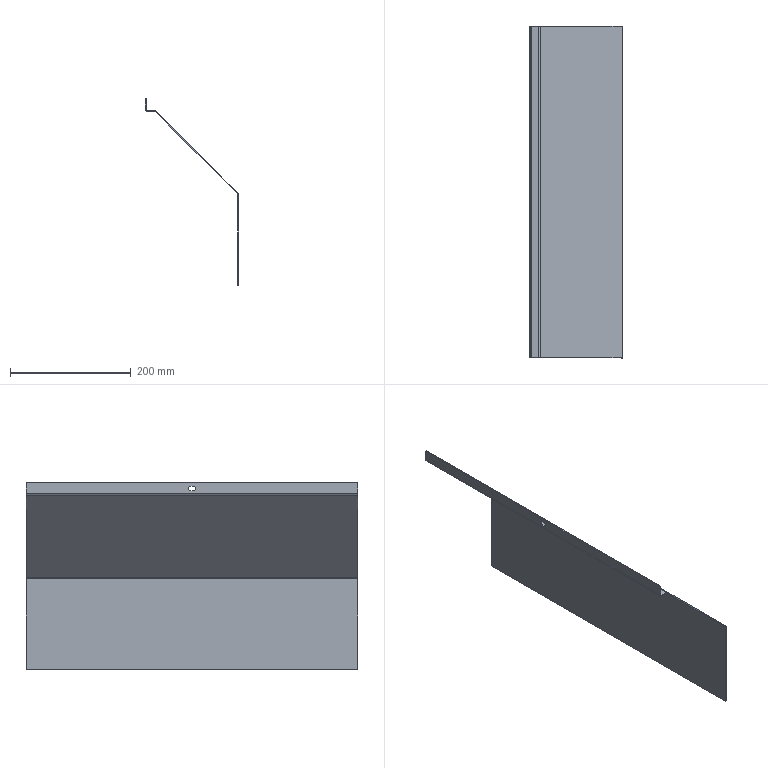Part | STEP file | SYL_0392D6J1SYL0380DJ100-939135 | 1 solid | 34 faces | box 155 x 550 x 310 mm | volume 314616 mm3 | plane 26 | cylinder 8 | commonest cylinder face diameters 4 x3 7 x3 8 x2
STEP:
#1=CARTESIAN_POINT('',(-1.5,-2.,14.));
#2=VERTEX_POINT('',#1);
#3=CARTESIAN_POINT('',(0.,-2.,14.));
#4=VERTEX_POINT('',#3);
#5=CARTESIAN_POINT('',(0.,-2.,14.));
#6=DIRECTION('',(1.,0.,0.));
#7=VECTOR('',#6,1000.);
#8=LINE('',#5,#7);
#9=EDGE_CURVE('',#2,#4,#8,.T.);
#10=ORIENTED_EDGE('',*,*,#9,.F.);
#11=CARTESIAN_POINT('',(-1.5,2.,14.));
#12=VERTEX_POINT('',#11);
#13=CARTESIAN_POINT('',(-1.5,-275.,14.));
#14=DIRECTION('',(0.,-1.,0.));
#15=VECTOR('',#14,1000.);
#16=LINE('',#13,#15);
#17=EDGE_CURVE('',#12,#2,#16,.T.);
#18=ORIENTED_EDGE('',*,*,#17,.F.);
#19=CARTESIAN_POINT('',(0.,2.,14.));
#20=VERTEX_POINT('',#19);
#21=CARTESIAN_POINT('',(0.,2.,14.));
#22=DIRECTION('',(1.,0.,0.));
#23=VECTOR('',#22,1000.);
#24=LINE('',#21,#23);
#25=EDGE_CURVE('',#12,#20,#24,.T.);
#26=ORIENTED_EDGE('',*,*,#25,.T.);
#27=CARTESIAN_POINT('',(0.,2.,14.));
#28=DIRECTION('',(0.,-1.,0.));
#29=VECTOR('',#28,1000.);
#30=LINE('',#27,#29);
#31=EDGE_CURVE('',#20,#4,#30,.T.);
#32=ORIENTED_EDGE('',*,*,#31,.T.);
#33=EDGE_LOOP('',(#10,#18,#26,#32));
#34=FACE_OUTER_BOUND('',#33,.T.);
#35=CARTESIAN_POINT('',(0.,2.,14.));
#36=DIRECTION('',(0.,0.,1.));
#37=DIRECTION('',(0.,-1.,0.));
#38=AXIS2_PLACEMENT_3D('',#35,#36,#37);
#39=PLANE('',#38);
#40=ADVANCED_FACE('',(#34),#39,.F.);
#41=ORIENTED_EDGE('',*,*,#25,.F.);
#42=CARTESIAN_POINT('',(-1.5,2.,6.));
#43=VERTEX_POINT('',#42);
#44=CARTESIAN_POINT('',(-1.5,2.,10.));
#45=DIRECTION('',(-1.,0.,0.));
#46=DIRECTION('',(0.,0.,1.));
#47=AXIS2_PLACEMENT_3D('',#44,#45,#46);
#48=CIRCLE('',#47,4.);
#49=EDGE_CURVE('',#12,#43,#48,.T.);
#50=ORIENTED_EDGE('',*,*,#49,.T.);
#51=CARTESIAN_POINT('',(0.,2.,6.));
#52=VERTEX_POINT('',#51);
#53=CARTESIAN_POINT('',(0.,2.,6.));
#54=DIRECTION('',(1.,0.,0.));
#55=VECTOR('',#54,1000.);
#56=LINE('',#53,#55);
#57=EDGE_CURVE('',#43,#52,#56,.T.);
#58=ORIENTED_EDGE('',*,*,#57,.T.);
#59=CARTESIAN_POINT('',(0.,2.,10.));
#60=DIRECTION('',(-1.,0.,0.));
#61=DIRECTION('',(0.,0.,1.));
#62=AXIS2_PLACEMENT_3D('',#59,#60,#61);
#63=CIRCLE('',#62,4.);
#64=EDGE_CURVE('',#20,#52,#63,.T.);
#65=ORIENTED_EDGE('',*,*,#64,.F.);
#66=EDGE_LOOP('',(#41,#50,#58,#65));
#67=FACE_OUTER_BOUND('',#66,.T.);
#68=CARTESIAN_POINT('',(0.,2.,10.));
#69=DIRECTION('',(1.,0.,0.));
#70=DIRECTION('',(0.,0.,-1.));
#71=AXIS2_PLACEMENT_3D('',#68,#69,#70);
#72=CYLINDRICAL_SURFACE('',#71,4.);
#73=ADVANCED_FACE('',(#67),#72,.F.);
#74=ORIENTED_EDGE('',*,*,#57,.F.);
#75=CARTESIAN_POINT('',(-1.5,-2.,6.));
#76=VERTEX_POINT('',#75);
#77=CARTESIAN_POINT('',(-1.5,-275.,6.));
#78=DIRECTION('',(0.,1.,0.));
#79=VECTOR('',#78,1000.);
#80=LINE('',#77,#79);
#81=EDGE_CURVE('',#76,#43,#80,.T.);
#82=ORIENTED_EDGE('',*,*,#81,.F.);
#83=CARTESIAN_POINT('',(0.,-2.,6.));
#84=VERTEX_POINT('',#83);
#85=CARTESIAN_POINT('',(0.,-2.,6.));
#86=DIRECTION('',(1.,0.,0.));
#87=VECTOR('',#86,1000.);
#88=LINE('',#85,#87);
#89=EDGE_CURVE('',#76,#84,#88,.T.);
#90=ORIENTED_EDGE('',*,*,#89,.T.);
#91=CARTESIAN_POINT('',(0.,-2.,6.));
#92=DIRECTION('',(0.,1.,0.));
#93=VECTOR('',#92,1000.);
#94=LINE('',#91,#93);
#95=EDGE_CURVE('',#84,#52,#94,.T.);
#96=ORIENTED_EDGE('',*,*,#95,.T.);
#97=EDGE_LOOP('',(#74,#82,#90,#96));
#98=FACE_OUTER_BOUND('',#97,.T.);
#99=CARTESIAN_POINT('',(0.,-2.,6.));
#100=DIRECTION('',(0.,0.,-1.));
#101=DIRECTION('',(0.,1.,0.));
#102=AXIS2_PLACEMENT_3D('',#99,#100,#101);
#103=PLANE('',#102);
#104=ADVANCED_FACE('',(#98),#103,.F.);
#105=CARTESIAN_POINT('',(14.05,-275.,-1.5));
#106=VERTEX_POINT('',#105);
#107=CARTESIAN_POINT('',(14.05,-275.,0.));
#108=VERTEX_POINT('',#107);
#109=CARTESIAN_POINT('',(14.05,-275.,0.));
#110=DIRECTION('',(0.,0.,1.));
#111=VECTOR('',#110,1000.);
#112=LINE('',#109,#111);
#113=EDGE_CURVE('',#106,#108,#112,.T.);
#114=ORIENTED_EDGE('',*,*,#113,.F.);
#115=CARTESIAN_POINT('',(15.464,-275.,-2.086));
#116=VERTEX_POINT('',#115);
#117=CARTESIAN_POINT('',(14.05,-275.,-3.5));
#118=DIRECTION('',(0.,-1.,0.));
#119=DIRECTION('',(0.,0.,-1.));
#120=AXIS2_PLACEMENT_3D('',#117,#118,#119);
#121=CIRCLE('',#120,2.);
#122=EDGE_CURVE('',#116,#106,#121,.T.);
#123=ORIENTED_EDGE('',*,*,#122,.F.);
#124=CARTESIAN_POINT('',(16.525,-275.,-1.025));
#125=VERTEX_POINT('',#124);
#126=CARTESIAN_POINT('',(16.525,-275.,-1.025));
#127=DIRECTION('',(0.7071,0.,0.7071));
#128=VECTOR('',#127,1000.);
#129=LINE('',#126,#128);
#130=EDGE_CURVE('',#116,#125,#129,.T.);
#131=ORIENTED_EDGE('',*,*,#130,.T.);
#132=CARTESIAN_POINT('',(14.05,-275.,-3.5));
#133=DIRECTION('',(0.,-1.,0.));
#134=DIRECTION('',(0.7071,0.,0.7071));
#135=AXIS2_PLACEMENT_3D('',#132,#133,#134);
#136=CIRCLE('',#135,3.5);
#137=EDGE_CURVE('',#125,#108,#136,.T.);
#138=ORIENTED_EDGE('',*,*,#137,.T.);
#139=EDGE_LOOP('',(#114,#123,#131,#138));
#140=FACE_OUTER_BOUND('',#139,.T.);
#141=CARTESIAN_POINT('',(14.05,-275.,-3.5));
#142=DIRECTION('',(0.,1.,0.));
#143=DIRECTION('',(0.,0.,1.));
#144=AXIS2_PLACEMENT_3D('',#141,#142,#143);
#145=PLANE('',#144);
#146=ADVANCED_FACE('',(#140),#145,.F.);
#147=ORIENTED_EDGE('',*,*,#130,.F.);
#148=CARTESIAN_POINT('',(151.414,-275.,-138.036));
#149=VERTEX_POINT('',#148);
#150=CARTESIAN_POINT('',(14.439,-275.,-1.061));
#151=DIRECTION('',(-0.7071,0.,0.7071));
#152=VECTOR('',#151,1000.);
#153=LINE('',#150,#152);
#154=EDGE_CURVE('',#149,#116,#153,.T.);
#155=ORIENTED_EDGE('',*,*,#154,.F.);
#156=CARTESIAN_POINT('',(152.475,-275.,-136.975));
#157=VERTEX_POINT('',#156);
#158=CARTESIAN_POINT('',(152.475,-275.,-136.975));
#159=DIRECTION('',(0.7071,0.,0.7071));
#160=VECTOR('',#159,1000.);
#161=LINE('',#158,#160);
#162=EDGE_CURVE('',#149,#157,#161,.T.);
#163=ORIENTED_EDGE('',*,*,#162,.T.);
#164=CARTESIAN_POINT('',(152.475,-275.,-136.975));
#165=DIRECTION('',(-0.7071,0.,0.7071));
#166=VECTOR('',#165,1000.);
#167=LINE('',#164,#166);
#168=EDGE_CURVE('',#157,#125,#167,.T.);
#169=ORIENTED_EDGE('',*,*,#168,.T.);
#170=EDGE_LOOP('',(#147,#155,#163,#169));
#171=FACE_OUTER_BOUND('',#170,.T.);
#172=CARTESIAN_POINT('',(152.475,-275.,-136.975));
#173=DIRECTION('',(0.,1.,0.));
#174=DIRECTION('',(-0.7071,0.,0.7071));
#175=AXIS2_PLACEMENT_3D('',#172,#173,#174);
#176=PLANE('',#175);
#177=ADVANCED_FACE('',(#171),#176,.F.);
#178=ORIENTED_EDGE('',*,*,#162,.F.);
#179=CARTESIAN_POINT('',(152.,-275.,-139.45));
#180=VERTEX_POINT('',#179);
#181=CARTESIAN_POINT('',(150.,-275.,-139.45));
#182=DIRECTION('',(0.,-1.,0.));
#183=DIRECTION('',(0.,0.,-1.));
#184=AXIS2_PLACEMENT_3D('',#181,#182,#183);
#185=CIRCLE('',#184,2.);
#186=EDGE_CURVE('',#180,#149,#185,.T.);
#187=ORIENTED_EDGE('',*,*,#186,.F.);
#188=CARTESIAN_POINT('',(153.5,-275.,-139.45));
#189=VERTEX_POINT('',#188);
#190=CARTESIAN_POINT('',(153.5,-275.,-139.45));
#191=DIRECTION('',(1.,0.,0.));
#192=VECTOR('',#191,1000.);
#193=LINE('',#190,#192);
#194=EDGE_CURVE('',#180,#189,#193,.T.);
#195=ORIENTED_EDGE('',*,*,#194,.T.);
#196=CARTESIAN_POINT('',(150.,-275.,-139.45));
#197=DIRECTION('',(0.,-1.,0.));
#198=DIRECTION('',(1.,0.,0.));
#199=AXIS2_PLACEMENT_3D('',#196,#197,#198);
#200=CIRCLE('',#199,3.5);
#201=EDGE_CURVE('',#189,#157,#200,.T.);
#202=ORIENTED_EDGE('',*,*,#201,.T.);
#203=EDGE_LOOP('',(#178,#187,#195,#202));
#204=FACE_OUTER_BOUND('',#203,.T.);
#205=CARTESIAN_POINT('',(150.,-275.,-139.45));
#206=DIRECTION('',(0.,1.,0.));
#207=DIRECTION('',(0.,0.,1.));
#208=AXIS2_PLACEMENT_3D('',#205,#206,#207);
#209=PLANE('',#208);
#210=ADVANCED_FACE('',(#204),#209,.F.);
#211=ORIENTED_EDGE('',*,*,#194,.F.);
#212=CARTESIAN_POINT('',(152.,-275.,-290.));
#213=VERTEX_POINT('',#212);
#214=CARTESIAN_POINT('',(152.,-275.,-138.));
#215=DIRECTION('',(0.,0.,1.));
#216=VECTOR('',#215,1000.);
#217=LINE('',#214,#216);
#218=EDGE_CURVE('',#213,#180,#217,.T.);
#219=ORIENTED_EDGE('',*,*,#218,.F.);
#220=CARTESIAN_POINT('',(153.5,-275.,-290.));
#221=VERTEX_POINT('',#220);
#222=CARTESIAN_POINT('',(153.5,-275.,-290.));
#223=DIRECTION('',(1.,0.,0.));
#224=VECTOR('',#223,1000.);
#225=LINE('',#222,#224);
#226=EDGE_CURVE('',#213,#221,#225,.T.);
#227=ORIENTED_EDGE('',*,*,#226,.T.);
#228=CARTESIAN_POINT('',(153.5,-275.,-290.));
#229=DIRECTION('',(0.,0.,1.));
#230=VECTOR('',#229,1000.);
#231=LINE('',#228,#230);
#232=EDGE_CURVE('',#221,#189,#231,.T.);
#233=ORIENTED_EDGE('',*,*,#232,.T.);
#234=EDGE_LOOP('',(#211,#219,#227,#233));
#235=FACE_OUTER_BOUND('',#234,.T.);
#236=CARTESIAN_POINT('',(153.5,-275.,-290.));
#237=DIRECTION('',(0.,1.,0.));
#238=DIRECTION('',(0.,0.,1.));
#239=AXIS2_PLACEMENT_3D('',#236,#237,#238);
#240=PLANE('',#239);
#241=ADVANCED_FACE('',(#235),#240,.F.);
#242=ORIENTED_EDGE('',*,*,#226,.F.);
#243=CARTESIAN_POINT('',(152.,275.,-290.));
#244=VERTEX_POINT('',#243);
#245=CARTESIAN_POINT('',(152.,-275.,-290.));
#246=DIRECTION('',(0.,-1.,0.));
#247=VECTOR('',#246,1000.);
#248=LINE('',#245,#247);
#249=EDGE_CURVE('',#244,#213,#248,.T.);
#250=ORIENTED_EDGE('',*,*,#249,.F.);
#251=CARTESIAN_POINT('',(153.5,275.,-290.));
#252=VERTEX_POINT('',#251);
#253=CARTESIAN_POINT('',(153.5,275.,-290.));
#254=DIRECTION('',(1.,0.,0.));
#255=VECTOR('',#254,1000.);
#256=LINE('',#253,#255);
#257=EDGE_CURVE('',#244,#252,#256,.T.);
#258=ORIENTED_EDGE('',*,*,#257,.T.);
#259=CARTESIAN_POINT('',(153.5,275.,-290.));
#260=DIRECTION('',(0.,-1.,0.));
#261=VECTOR('',#260,1000.);
#262=LINE('',#259,#261);
#263=EDGE_CURVE('',#252,#221,#262,.T.);
#264=ORIENTED_EDGE('',*,*,#263,.T.);
#265=EDGE_LOOP('',(#242,#250,#258,#264));
#266=FACE_OUTER_BOUND('',#265,.T.);
#267=CARTESIAN_POINT('',(153.5,275.,-290.));
#268=DIRECTION('',(0.,0.,1.));
#269=DIRECTION('',(0.,-1.,0.));
#270=AXIS2_PLACEMENT_3D('',#267,#268,#269);
#271=PLANE('',#270);
#272=ADVANCED_FACE('',(#266),#271,.F.);
#273=ORIENTED_EDGE('',*,*,#257,.F.);
#274=CARTESIAN_POINT('',(152.,275.,-139.45));
#275=VERTEX_POINT('',#274);
#276=CARTESIAN_POINT('',(152.,275.,-138.));
#277=DIRECTION('',(0.,0.,-1.));
#278=VECTOR('',#277,1000.);
#279=LINE('',#276,#278);
#280=EDGE_CURVE('',#275,#244,#279,.T.);
#281=ORIENTED_EDGE('',*,*,#280,.F.);
#282=CARTESIAN_POINT('',(153.5,275.,-139.45));
#283=VERTEX_POINT('',#282);
#284=CARTESIAN_POINT('',(153.5,275.,-139.45));
#285=DIRECTION('',(1.,0.,0.));
#286=VECTOR('',#285,1000.);
#287=LINE('',#284,#286);
#288=EDGE_CURVE('',#275,#283,#287,.T.);
#289=ORIENTED_EDGE('',*,*,#288,.T.);
#290=CARTESIAN_POINT('',(153.5,275.,-139.45));
#291=DIRECTION('',(0.,0.,-1.));
#292=VECTOR('',#291,1000.);
#293=LINE('',#290,#292);
#294=EDGE_CURVE('',#283,#252,#293,.T.);
#295=ORIENTED_EDGE('',*,*,#294,.T.);
#296=EDGE_LOOP('',(#273,#281,#289,#295));
#297=FACE_OUTER_BOUND('',#296,.T.);
#298=CARTESIAN_POINT('',(153.5,275.,-139.45));
#299=DIRECTION('',(0.,-1.,0.));
#300=DIRECTION('',(0.,0.,-1.));
#301=AXIS2_PLACEMENT_3D('',#298,#299,#300);
#302=PLANE('',#301);
#303=ADVANCED_FACE('',(#297),#302,.F.);
#304=ORIENTED_EDGE('',*,*,#288,.F.);
#305=CARTESIAN_POINT('',(151.414,275.,-138.036));
#306=VERTEX_POINT('',#305);
#307=CARTESIAN_POINT('',(150.,275.,-139.45));
#308=DIRECTION('',(0.,1.,0.));
#309=DIRECTION('',(0.,0.,-1.));
#310=AXIS2_PLACEMENT_3D('',#307,#308,#309);
#311=CIRCLE('',#310,2.);
#312=EDGE_CURVE('',#306,#275,#311,.T.);
#313=ORIENTED_EDGE('',*,*,#312,.F.);
#314=CARTESIAN_POINT('',(152.475,275.,-136.975));
#315=VERTEX_POINT('',#314);
#316=CARTESIAN_POINT('',(152.475,275.,-136.975));
#317=DIRECTION('',(0.7071,0.,0.7071));
#318=VECTOR('',#317,1000.);
#319=LINE('',#316,#318);
#320=EDGE_CURVE('',#306,#315,#319,.T.);
#321=ORIENTED_EDGE('',*,*,#320,.T.);
#322=CARTESIAN_POINT('',(150.,275.,-139.45));
#323=DIRECTION('',(0.,1.,0.));
#324=DIRECTION('',(0.7071,0.,0.7071));
#325=AXIS2_PLACEMENT_3D('',#322,#323,#324);
#326=CIRCLE('',#325,3.5);
#327=EDGE_CURVE('',#315,#283,#326,.T.);
#328=ORIENTED_EDGE('',*,*,#327,.T.);
#329=EDGE_LOOP('',(#304,#313,#321,#328));
#330=FACE_OUTER_BOUND('',#329,.T.);
#331=CARTESIAN_POINT('',(150.,275.,-139.45));
#332=DIRECTION('',(0.,-1.,0.));
#333=DIRECTION('',(0.,0.,-1.));
#334=AXIS2_PLACEMENT_3D('',#331,#332,#333);
#335=PLANE('',#334);
#336=ADVANCED_FACE('',(#330),#335,.F.);
#337=ORIENTED_EDGE('',*,*,#320,.F.);
#338=CARTESIAN_POINT('',(15.464,275.,-2.086));
#339=VERTEX_POINT('',#338);
#340=CARTESIAN_POINT('',(14.439,275.,-1.061));
#341=DIRECTION('',(0.7071,0.,-0.7071));
#342=VECTOR('',#341,1000.);
#343=LINE('',#340,#342);
#344=EDGE_CURVE('',#339,#306,#343,.T.);
#345=ORIENTED_EDGE('',*,*,#344,.F.);
#346=CARTESIAN_POINT('',(16.525,275.,-1.025));
#347=VERTEX_POINT('',#346);
#348=CARTESIAN_POINT('',(16.525,275.,-1.025));
#349=DIRECTION('',(0.7071,0.,0.7071));
#350=VECTOR('',#349,1000.);
#351=LINE('',#348,#350);
#352=EDGE_CURVE('',#339,#347,#351,.T.);
#353=ORIENTED_EDGE('',*,*,#352,.T.);
#354=CARTESIAN_POINT('',(16.525,275.,-1.025));
#355=DIRECTION('',(0.7071,0.,-0.7071));
#356=VECTOR('',#355,1000.);
#357=LINE('',#354,#356);
#358=EDGE_CURVE('',#347,#315,#357,.T.);
#359=ORIENTED_EDGE('',*,*,#358,.T.);
#360=EDGE_LOOP('',(#337,#345,#353,#359));
#361=FACE_OUTER_BOUND('',#360,.T.);
#362=CARTESIAN_POINT('',(16.525,275.,-1.025));
#363=DIRECTION('',(0.,-1.,0.));
#364=DIRECTION('',(0.7071,0.,-0.7071));
#365=AXIS2_PLACEMENT_3D('',#362,#363,#364);
#366=PLANE('',#365);
#367=ADVANCED_FACE('',(#361),#366,.F.);
#368=ORIENTED_EDGE('',*,*,#352,.F.);
#369=CARTESIAN_POINT('',(14.05,275.,-1.5));
#370=VERTEX_POINT('',#369);
#371=CARTESIAN_POINT('',(14.05,275.,-3.5));
#372=DIRECTION('',(0.,1.,0.));
#373=DIRECTION('',(0.,0.,-1.));
#374=AXIS2_PLACEMENT_3D('',#371,#372,#373);
#375=CIRCLE('',#374,2.);
#376=EDGE_CURVE('',#370,#339,#375,.T.);
#377=ORIENTED_EDGE('',*,*,#376,.F.);
#378=CARTESIAN_POINT('',(14.05,275.,0.));
#379=VERTEX_POINT('',#378);
#380=CARTESIAN_POINT('',(14.05,275.,0.));
#381=DIRECTION('',(0.,0.,1.));
#382=VECTOR('',#381,1000.);
#383=LINE('',#380,#382);
#384=EDGE_CURVE('',#370,#379,#383,.T.);
#385=ORIENTED_EDGE('',*,*,#384,.T.);
#386=CARTESIAN_POINT('',(14.05,275.,-3.5));
#387=DIRECTION('',(0.,1.,0.));
#388=DIRECTION('',(0.,0.,1.));
#389=AXIS2_PLACEMENT_3D('',#386,#387,#388);
#390=CIRCLE('',#389,3.5);
#391=EDGE_CURVE('',#379,#347,#390,.T.);
#392=ORIENTED_EDGE('',*,*,#391,.T.);
#393=EDGE_LOOP('',(#368,#377,#385,#392));
#394=FACE_OUTER_BOUND('',#393,.T.);
#395=CARTESIAN_POINT('',(14.05,275.,-3.5));
#396=DIRECTION('',(0.,-1.,0.));
#397=DIRECTION('',(0.,0.,-1.));
#398=AXIS2_PLACEMENT_3D('',#395,#396,#397);
#399=PLANE('',#398);
#400=ADVANCED_FACE('',(#394),#399,.F.);
#401=ORIENTED_EDGE('',*,*,#384,.F.);
#402=CARTESIAN_POINT('',(2.,275.,-1.5));
#403=VERTEX_POINT('',#402);
#404=CARTESIAN_POINT('',(0.,275.,-1.5));
#405=DIRECTION('',(1.,0.,0.));
#406=VECTOR('',#405,1000.);
#407=LINE('',#404,#406);
#408=EDGE_CURVE('',#403,#370,#407,.T.);
#409=ORIENTED_EDGE('',*,*,#408,.F.);
#410=CARTESIAN_POINT('',(2.,275.,0.));
#411=VERTEX_POINT('',#410);
#412=CARTESIAN_POINT('',(2.,275.,0.));
#413=DIRECTION('',(0.,0.,1.));
#414=VECTOR('',#413,1000.);
#415=LINE('',#412,#414);
#416=EDGE_CURVE('',#403,#411,#415,.T.);
#417=ORIENTED_EDGE('',*,*,#416,.T.);
#418=CARTESIAN_POINT('',(2.,275.,0.));
#419=DIRECTION('',(1.,0.,0.));
#420=VECTOR('',#419,1000.);
#421=LINE('',#418,#420);
#422=EDGE_CURVE('',#411,#379,#421,.T.);
#423=ORIENTED_EDGE('',*,*,#422,.T.);
#424=EDGE_LOOP('',(#401,#409,#417,#423));
#425=FACE_OUTER_BOUND('',#424,.T.);
#426=CARTESIAN_POINT('',(2.,275.,0.));
#427=DIRECTION('',(0.,-1.,0.));
#428=DIRECTION('',(1.,0.,0.));
#429=AXIS2_PLACEMENT_3D('',#426,#427,#428);
#430=PLANE('',#429);
#431=ADVANCED_FACE('',(#425),#430,.F.);
#432=ORIENTED_EDGE('',*,*,#416,.F.);
#433=CARTESIAN_POINT('',(-1.5,275.,2.));
#434=VERTEX_POINT('',#433);
#435=CARTESIAN_POINT('',(2.,275.,2.));
#436=DIRECTION('',(0.,-1.,0.));
#437=DIRECTION('',(0.,0.,1.));
#438=AXIS2_PLACEMENT_3D('',#435,#436,#437);
#439=CIRCLE('',#438,3.5);
#440=EDGE_CURVE('',#434,#403,#439,.T.);
#441=ORIENTED_EDGE('',*,*,#440,.F.);
#442=CARTESIAN_POINT('',(0.,275.,2.));
#443=VERTEX_POINT('',#442);
#444=CARTESIAN_POINT('',(0.,275.,2.));
#445=DIRECTION('',(1.,0.,0.));
#446=VECTOR('',#445,1000.);
#447=LINE('',#444,#446);
#448=EDGE_CURVE('',#434,#443,#447,.T.);
#449=ORIENTED_EDGE('',*,*,#448,.T.);
#450=CARTESIAN_POINT('',(2.,275.,2.));
#451=DIRECTION('',(0.,-1.,0.));
#452=DIRECTION('',(-1.,0.,0.));
#453=AXIS2_PLACEMENT_3D('',#450,#451,#452);
#454=CIRCLE('',#453,2.);
#455=EDGE_CURVE('',#443,#411,#454,.T.);
#456=ORIENTED_EDGE('',*,*,#455,.T.);
#457=EDGE_LOOP('',(#432,#441,#449,#456));
#458=FACE_OUTER_BOUND('',#457,.T.);
#459=CARTESIAN_POINT('',(2.,275.,2.));
#460=DIRECTION('',(0.,1.,0.));
#461=DIRECTION('',(0.,0.,1.));
#462=AXIS2_PLACEMENT_3D('',#459,#460,#461);
#463=PLANE('',#462);
#464=ADVANCED_FACE('',(#458),#463,.T.);
#465=ORIENTED_EDGE('',*,*,#448,.F.);
#466=CARTESIAN_POINT('',(-1.5,275.,20.));
#467=VERTEX_POINT('',#466);
#468=CARTESIAN_POINT('',(-1.5,275.,20.));
#469=DIRECTION('',(0.,0.,-1.));
#470=VECTOR('',#469,1000.);
#471=LINE('',#468,#470);
#472=EDGE_CURVE('',#467,#434,#471,.T.);
#473=ORIENTED_EDGE('',*,*,#472,.F.);
#474=CARTESIAN_POINT('',(0.,275.,20.));
#475=VERTEX_POINT('',#474);
#476=CARTESIAN_POINT('',(0.,275.,20.));
#477=DIRECTION('',(1.,0.,0.));
#478=VECTOR('',#477,1000.);
#479=LINE('',#476,#478);
#480=EDGE_CURVE('',#467,#475,#479,.T.);
#481=ORIENTED_EDGE('',*,*,#480,.T.);
#482=CARTESIAN_POINT('',(0.,275.,20.));
#483=DIRECTION('',(0.,0.,-1.));
#484=VECTOR('',#483,1000.);
#485=LINE('',#482,#484);
#486=EDGE_CURVE('',#475,#443,#485,.T.);
#487=ORIENTED_EDGE('',*,*,#486,.T.);
#488=EDGE_LOOP('',(#465,#473,#481,#487));
#489=FACE_OUTER_BOUND('',#488,.T.);
#490=CARTESIAN_POINT('',(0.,275.,20.));
#491=DIRECTION('',(0.,-1.,0.));
#492=DIRECTION('',(0.,0.,-1.));
#493=AXIS2_PLACEMENT_3D('',#490,#491,#492);
#494=PLANE('',#493);
#495=ADVANCED_FACE('',(#489),#494,.F.);
#496=ORIENTED_EDGE('',*,*,#480,.F.);
#497=CARTESIAN_POINT('',(-1.5,-275.,20.));
#498=VERTEX_POINT('',#497);
#499=CARTESIAN_POINT('',(-1.5,-275.,20.));
#500=DIRECTION('',(0.,1.,0.));
#501=VECTOR('',#500,1000.);
#502=LINE('',#499,#501);
#503=EDGE_CURVE('',#498,#467,#502,.T.);
#504=ORIENTED_EDGE('',*,*,#503,.F.);
#505=CARTESIAN_POINT('',(0.,-275.,20.));
#506=VERTEX_POINT('',#505);
#507=CARTESIAN_POINT('',(0.,-275.,20.));
#508=DIRECTION('',(1.,0.,0.));
#509=VECTOR('',#508,1000.);
#510=LINE('',#507,#509);
#511=EDGE_CURVE('',#498,#506,#510,.T.);
#512=ORIENTED_EDGE('',*,*,#511,.T.);
#513=CARTESIAN_POINT('',(0.,-275.,20.));
#514=DIRECTION('',(0.,1.,0.));
#515=VECTOR('',#514,1000.);
#516=LINE('',#513,#515);
#517=EDGE_CURVE('',#506,#475,#516,.T.);
#518=ORIENTED_EDGE('',*,*,#517,.T.);
#519=EDGE_LOOP('',(#496,#504,#512,#518));
#520=FACE_OUTER_BOUND('',#519,.T.);
#521=CARTESIAN_POINT('',(0.,-275.,20.));
#522=DIRECTION('',(0.,0.,-1.));
#523=DIRECTION('',(0.,1.,0.));
#524=AXIS2_PLACEMENT_3D('',#521,#522,#523);
#525=PLANE('',#524);
#526=ADVANCED_FACE('',(#520),#525,.F.);
#527=ORIENTED_EDGE('',*,*,#511,.F.);
#528=CARTESIAN_POINT('',(-1.5,-275.,2.));
#529=VERTEX_POINT('',#528);
#530=CARTESIAN_POINT('',(-1.5,-275.,20.));
#531=DIRECTION('',(0.,0.,1.));
#532=VECTOR('',#531,1000.);
#533=LINE('',#530,#532);
#534=EDGE_CURVE('',#529,#498,#533,.T.);
#535=ORIENTED_EDGE('',*,*,#534,.F.);
#536=CARTESIAN_POINT('',(0.,-275.,2.));
#537=VERTEX_POINT('',#536);
#538=CARTESIAN_POINT('',(0.,-275.,2.));
#539=DIRECTION('',(1.,0.,0.));
#540=VECTOR('',#539,1000.);
#541=LINE('',#538,#540);
#542=EDGE_CURVE('',#529,#537,#541,.T.);
#543=ORIENTED_EDGE('',*,*,#542,.T.);
#544=CARTESIAN_POINT('',(0.,-275.,2.));
#545=DIRECTION('',(0.,0.,1.));
#546=VECTOR('',#545,1000.);
#547=LINE('',#544,#546);
#548=EDGE_CURVE('',#537,#506,#547,.T.);
#549=ORIENTED_EDGE('',*,*,#548,.T.);
#550=EDGE_LOOP('',(#527,#535,#543,#549));
#551=FACE_OUTER_BOUND('',#550,.T.);
#552=CARTESIAN_POINT('',(0.,-275.,2.));
#553=DIRECTION('',(0.,1.,0.));
#554=DIRECTION('',(0.,0.,1.));
#555=AXIS2_PLACEMENT_3D('',#552,#553,#554);
#556=PLANE('',#555);
#557=ADVANCED_FACE('',(#551),#556,.F.);
#558=ORIENTED_EDGE('',*,*,#542,.F.);
#559=CARTESIAN_POINT('',(2.,-275.,-1.5));
#560=VERTEX_POINT('',#559);
#561=CARTESIAN_POINT('',(2.,-275.,2.));
#562=DIRECTION('',(0.,1.,0.));
#563=DIRECTION('',(0.,0.,1.));
#564=AXIS2_PLACEMENT_3D('',#561,#562,#563);
#565=CIRCLE('',#564,3.5);
#566=EDGE_CURVE('',#560,#529,#565,.T.);
#567=ORIENTED_EDGE('',*,*,#566,.F.);
#568=CARTESIAN_POINT('',(2.,-275.,0.));
#569=VERTEX_POINT('',#568);
#570=CARTESIAN_POINT('',(2.,-275.,0.));
#571=DIRECTION('',(0.,0.,1.));
#572=VECTOR('',#571,1000.);
#573=LINE('',#570,#572);
#574=EDGE_CURVE('',#560,#569,#573,.T.);
#575=ORIENTED_EDGE('',*,*,#574,.T.);
#576=CARTESIAN_POINT('',(2.,-275.,2.));
#577=DIRECTION('',(0.,1.,0.));
#578=DIRECTION('',(0.,0.,-1.));
#579=AXIS2_PLACEMENT_3D('',#576,#577,#578);
#580=CIRCLE('',#579,2.);
#581=EDGE_CURVE('',#569,#537,#580,.T.);
#582=ORIENTED_EDGE('',*,*,#581,.T.);
#583=EDGE_LOOP('',(#558,#567,#575,#582));
#584=FACE_OUTER_BOUND('',#583,.T.);
#585=CARTESIAN_POINT('',(2.,-275.,2.));
#586=DIRECTION('',(0.,-1.,0.));
#587=DIRECTION('',(0.,0.,-1.));
#588=AXIS2_PLACEMENT_3D('',#585,#586,#587);
#589=PLANE('',#588);
#590=ADVANCED_FACE('',(#584),#589,.T.);
#591=CARTESIAN_POINT('',(-1.5,-2.,10.));
#592=DIRECTION('',(-1.,0.,0.));
#593=DIRECTION('',(0.,0.,1.));
#594=AXIS2_PLACEMENT_3D('',#591,#592,#593);
#595=CIRCLE('',#594,4.);
#596=EDGE_CURVE('',#76,#2,#595,.T.);
#597=ORIENTED_EDGE('',*,*,#596,.T.);
#598=ORIENTED_EDGE('',*,*,#9,.T.);
#599=CARTESIAN_POINT('',(0.,-2.,10.));
#600=DIRECTION('',(-1.,0.,0.));
#601=DIRECTION('',(0.,0.,-1.));
#602=AXIS2_PLACEMENT_3D('',#599,#600,#601);
#603=CIRCLE('',#602,4.);
#604=EDGE_CURVE('',#84,#4,#603,.T.);
#605=ORIENTED_EDGE('',*,*,#604,.F.);
#606=ORIENTED_EDGE('',*,*,#89,.F.);
#607=EDGE_LOOP('',(#597,#598,#605,#606));
#608=FACE_OUTER_BOUND('',#607,.T.);
#609=CARTESIAN_POINT('',(0.,-2.,10.));
#610=DIRECTION('',(1.,0.,0.));
#611=DIRECTION('',(0.,0.,-1.));
#612=AXIS2_PLACEMENT_3D('',#609,#610,#611);
#613=CYLINDRICAL_SURFACE('',#612,4.);
#614=ADVANCED_FACE('',(#608),#613,.F.);
#615=CARTESIAN_POINT('',(0.,-275.,-1.5));
#616=DIRECTION('',(-1.,0.,0.));
#617=VECTOR('',#616,1000.);
#618=LINE('',#615,#617);
#619=EDGE_CURVE('',#106,#560,#618,.T.);
#620=ORIENTED_EDGE('',*,*,#619,.F.);
#621=ORIENTED_EDGE('',*,*,#113,.T.);
#622=CARTESIAN_POINT('',(14.05,-275.,0.));
#623=DIRECTION('',(-1.,0.,0.));
#624=VECTOR('',#623,1000.);
#625=LINE('',#622,#624);
#626=EDGE_CURVE('',#108,#569,#625,.T.);
#627=ORIENTED_EDGE('',*,*,#626,.T.);
#628=ORIENTED_EDGE('',*,*,#574,.F.);
#629=EDGE_LOOP('',(#620,#621,#627,#628));
#630=FACE_OUTER_BOUND('',#629,.T.);
#631=CARTESIAN_POINT('',(14.05,-275.,0.));
#632=DIRECTION('',(0.,1.,0.));
#633=DIRECTION('',(-1.,0.,0.));
#634=AXIS2_PLACEMENT_3D('',#631,#632,#633);
#635=PLANE('',#634);
#636=ADVANCED_FACE('',(#630),#635,.F.);
#637=ORIENTED_EDGE('',*,*,#581,.F.);
#638=CARTESIAN_POINT('',(2.,-275.,0.));
#639=DIRECTION('',(0.,1.,0.));
#640=VECTOR('',#639,1000.);
#641=LINE('',#638,#640);
#642=EDGE_CURVE('',#569,#411,#641,.T.);
#643=ORIENTED_EDGE('',*,*,#642,.T.);
#644=ORIENTED_EDGE('',*,*,#455,.F.);
#645=CARTESIAN_POINT('',(0.,275.,2.));
#646=DIRECTION('',(0.,-1.,0.));
#647=VECTOR('',#646,1000.);
#648=LINE('',#645,#647);
#649=EDGE_CURVE('',#443,#537,#648,.T.);
#650=ORIENTED_EDGE('',*,*,#649,.T.);
#651=EDGE_LOOP('',(#637,#643,#644,#650));
#652=FACE_OUTER_BOUND('',#651,.T.);
#653=CARTESIAN_POINT('',(2.,-275.,2.));
#654=DIRECTION('',(0.,1.,0.));
#655=DIRECTION('',(0.,0.,1.));
#656=AXIS2_PLACEMENT_3D('',#653,#654,#655);
#657=CYLINDRICAL_SURFACE('',#656,2.);
#658=ADVANCED_FACE('',(#652),#657,.F.);
#659=ORIENTED_EDGE('',*,*,#95,.F.);
#660=ORIENTED_EDGE('',*,*,#604,.T.);
#661=ORIENTED_EDGE('',*,*,#31,.F.);
#662=ORIENTED_EDGE('',*,*,#64,.T.);
#663=EDGE_LOOP('',(#659,#660,#661,#662));
#664=FACE_BOUND('',#663,.T.);
#665=ORIENTED_EDGE('',*,*,#548,.F.);
#666=ORIENTED_EDGE('',*,*,#649,.F.);
#667=ORIENTED_EDGE('',*,*,#486,.F.);
#668=ORIENTED_EDGE('',*,*,#517,.F.);
#669=EDGE_LOOP('',(#665,#666,#667,#668));
#670=FACE_OUTER_BOUND('',#669,.T.);
#671=CARTESIAN_POINT('',(0.,-275.,20.));
#672=DIRECTION('',(1.,0.,0.));
#673=DIRECTION('',(0.,1.,0.));
#674=AXIS2_PLACEMENT_3D('',#671,#672,#673);
#675=PLANE('',#674);
#676=ADVANCED_FACE('',(#664,#670),#675,.T.);
#677=CARTESIAN_POINT('',(16.525,-275.,-1.025));
#678=DIRECTION('',(0.,1.,0.));
#679=VECTOR('',#678,1000.);
#680=LINE('',#677,#679);
#681=EDGE_CURVE('',#125,#347,#680,.T.);
#682=ORIENTED_EDGE('',*,*,#681,.T.);
#683=ORIENTED_EDGE('',*,*,#391,.F.);
#684=CARTESIAN_POINT('',(14.05,275.,0.));
#685=DIRECTION('',(0.,-1.,0.));
#686=VECTOR('',#685,1000.);
#687=LINE('',#684,#686);
#688=EDGE_CURVE('',#379,#108,#687,.T.);
#689=ORIENTED_EDGE('',*,*,#688,.T.);
#690=ORIENTED_EDGE('',*,*,#137,.F.);
#691=EDGE_LOOP('',(#682,#683,#689,#690));
#692=FACE_OUTER_BOUND('',#691,.T.);
#693=CARTESIAN_POINT('',(14.05,-275.,-3.5));
#694=DIRECTION('',(0.,-1.,0.));
#695=DIRECTION('',(0.,0.,-1.));
#696=AXIS2_PLACEMENT_3D('',#693,#694,#695);
#697=CYLINDRICAL_SURFACE('',#696,3.5);
#698=ADVANCED_FACE('',(#692),#697,.T.);
#699=ORIENTED_EDGE('',*,*,#626,.F.);
#700=ORIENTED_EDGE('',*,*,#688,.F.);
#701=ORIENTED_EDGE('',*,*,#422,.F.);
#702=ORIENTED_EDGE('',*,*,#642,.F.);
#703=EDGE_LOOP('',(#699,#700,#701,#702));
#704=FACE_OUTER_BOUND('',#703,.T.);
#705=CARTESIAN_POINT('',(0.,-275.,0.));
#706=DIRECTION('',(0.,0.,1.));
#707=DIRECTION('',(1.,0.,0.));
#708=AXIS2_PLACEMENT_3D('',#705,#706,#707);
#709=PLANE('',#708);
#710=ADVANCED_FACE('',(#704),#709,.T.);
#711=CARTESIAN_POINT('',(153.5,-275.,-139.45));
#712=DIRECTION('',(0.,1.,0.));
#713=VECTOR('',#712,1000.);
#714=LINE('',#711,#713);
#715=EDGE_CURVE('',#189,#283,#714,.T.);
#716=ORIENTED_EDGE('',*,*,#715,.T.);
#717=ORIENTED_EDGE('',*,*,#327,.F.);
#718=CARTESIAN_POINT('',(152.475,275.,-136.975));
#719=DIRECTION('',(0.,-1.,0.));
#720=VECTOR('',#719,1000.);
#721=LINE('',#718,#720);
#722=EDGE_CURVE('',#315,#157,#721,.T.);
#723=ORIENTED_EDGE('',*,*,#722,.T.);
#724=ORIENTED_EDGE('',*,*,#201,.F.);
#725=EDGE_LOOP('',(#716,#717,#723,#724));
#726=FACE_OUTER_BOUND('',#725,.T.);
#727=CARTESIAN_POINT('',(150.,-275.,-139.45));
#728=DIRECTION('',(0.,-1.,0.));
#729=DIRECTION('',(0.,0.,-1.));
#730=AXIS2_PLACEMENT_3D('',#727,#728,#729);
#731=CYLINDRICAL_SURFACE('',#730,3.5);
#732=ADVANCED_FACE('',(#726),#731,.T.);
#733=ORIENTED_EDGE('',*,*,#168,.F.);
#734=ORIENTED_EDGE('',*,*,#722,.F.);
#735=ORIENTED_EDGE('',*,*,#358,.F.);
#736=ORIENTED_EDGE('',*,*,#681,.F.);
#737=EDGE_LOOP('',(#733,#734,#735,#736));
#738=FACE_OUTER_BOUND('',#737,.T.);
#739=CARTESIAN_POINT('',(15.5,-275.,0.));
#740=DIRECTION('',(0.7071,0.,0.7071));
#741=DIRECTION('',(0.,-1.,0.));
#742=AXIS2_PLACEMENT_3D('',#739,#740,#741);
#743=PLANE('',#742);
#744=ADVANCED_FACE('',(#738),#743,.T.);
#745=ORIENTED_EDGE('',*,*,#232,.F.);
#746=ORIENTED_EDGE('',*,*,#263,.F.);
#747=ORIENTED_EDGE('',*,*,#294,.F.);
#748=ORIENTED_EDGE('',*,*,#715,.F.);
#749=EDGE_LOOP('',(#745,#746,#747,#748));
#750=FACE_OUTER_BOUND('',#749,.T.);
#751=CARTESIAN_POINT('',(153.5,-275.,-138.));
#752=DIRECTION('',(1.,0.,0.));
#753=DIRECTION('',(0.,1.,0.));
#754=AXIS2_PLACEMENT_3D('',#751,#752,#753);
#755=PLANE('',#754);
#756=ADVANCED_FACE('',(#750),#755,.T.);
#757=ORIENTED_EDGE('',*,*,#566,.T.);
#758=CARTESIAN_POINT('',(-1.5,-275.,2.));
#759=DIRECTION('',(0.,-1.,0.));
#760=VECTOR('',#759,1000.);
#761=LINE('',#758,#760);
#762=EDGE_CURVE('',#434,#529,#761,.T.);
#763=ORIENTED_EDGE('',*,*,#762,.F.);
#764=ORIENTED_EDGE('',*,*,#440,.T.);
#765=CARTESIAN_POINT('',(2.,-275.,-1.5));
#766=DIRECTION('',(0.,1.,0.));
#767=VECTOR('',#766,1000.);
#768=LINE('',#765,#767);
#769=EDGE_CURVE('',#560,#403,#768,.T.);
#770=ORIENTED_EDGE('',*,*,#769,.F.);
#771=EDGE_LOOP('',(#757,#763,#764,#770));
#772=FACE_OUTER_BOUND('',#771,.T.);
#773=CARTESIAN_POINT('',(2.,-275.,2.));
#774=DIRECTION('',(0.,1.,0.));
#775=DIRECTION('',(0.,0.,1.));
#776=AXIS2_PLACEMENT_3D('',#773,#774,#775);
#777=CYLINDRICAL_SURFACE('',#776,3.5);
#778=ADVANCED_FACE('',(#772),#777,.T.);
#779=ORIENTED_EDGE('',*,*,#81,.T.);
#780=ORIENTED_EDGE('',*,*,#49,.F.);
#781=ORIENTED_EDGE('',*,*,#17,.T.);
#782=ORIENTED_EDGE('',*,*,#596,.F.);
#783=EDGE_LOOP('',(#779,#780,#781,#782));
#784=FACE_BOUND('',#783,.T.);
#785=ORIENTED_EDGE('',*,*,#534,.T.);
#786=ORIENTED_EDGE('',*,*,#503,.T.);
#787=ORIENTED_EDGE('',*,*,#472,.T.);
#788=ORIENTED_EDGE('',*,*,#762,.T.);
#789=EDGE_LOOP('',(#785,#786,#787,#788));
#790=FACE_OUTER_BOUND('',#789,.T.);
#791=CARTESIAN_POINT('',(-1.5,-275.,20.));
#792=DIRECTION('',(1.,0.,0.));
#793=DIRECTION('',(0.,1.,0.));
#794=AXIS2_PLACEMENT_3D('',#791,#792,#793);
#795=PLANE('',#794);
#796=ADVANCED_FACE('',(#784,#790),#795,.F.);
#797=CARTESIAN_POINT('',(15.464,-275.,-2.086));
#798=DIRECTION('',(0.,1.,0.));
#799=VECTOR('',#798,1000.);
#800=LINE('',#797,#799);
#801=EDGE_CURVE('',#116,#339,#800,.T.);
#802=ORIENTED_EDGE('',*,*,#801,.F.);
#803=ORIENTED_EDGE('',*,*,#122,.T.);
#804=CARTESIAN_POINT('',(14.05,-275.,-1.5));
#805=DIRECTION('',(0.,-1.,0.));
#806=VECTOR('',#805,1000.);
#807=LINE('',#804,#806);
#808=EDGE_CURVE('',#370,#106,#807,.T.);
#809=ORIENTED_EDGE('',*,*,#808,.F.);
#810=ORIENTED_EDGE('',*,*,#376,.T.);
#811=EDGE_LOOP('',(#802,#803,#809,#810));
#812=FACE_OUTER_BOUND('',#811,.T.);
#813=CARTESIAN_POINT('',(14.05,-275.,-3.5));
#814=DIRECTION('',(0.,-1.,0.));
#815=DIRECTION('',(0.,0.,-1.));
#816=AXIS2_PLACEMENT_3D('',#813,#814,#815);
#817=CYLINDRICAL_SURFACE('',#816,2.);
#818=ADVANCED_FACE('',(#812),#817,.F.);
#819=ORIENTED_EDGE('',*,*,#619,.T.);
#820=ORIENTED_EDGE('',*,*,#769,.T.);
#821=ORIENTED_EDGE('',*,*,#408,.T.);
#822=ORIENTED_EDGE('',*,*,#808,.T.);
#823=EDGE_LOOP('',(#819,#820,#821,#822));
#824=FACE_OUTER_BOUND('',#823,.T.);
#825=CARTESIAN_POINT('',(0.,-275.,-1.5));
#826=DIRECTION('',(0.,0.,1.));
#827=DIRECTION('',(1.,0.,0.));
#828=AXIS2_PLACEMENT_3D('',#825,#826,#827);
#829=PLANE('',#828);
#830=ADVANCED_FACE('',(#824),#829,.F.);
#831=CARTESIAN_POINT('',(152.,-275.,-139.45));
#832=DIRECTION('',(0.,1.,0.));
#833=VECTOR('',#832,1000.);
#834=LINE('',#831,#833);
#835=EDGE_CURVE('',#180,#275,#834,.T.);
#836=ORIENTED_EDGE('',*,*,#835,.F.);
#837=ORIENTED_EDGE('',*,*,#186,.T.);
#838=CARTESIAN_POINT('',(151.414,-275.,-138.036));
#839=DIRECTION('',(0.,-1.,0.));
#840=VECTOR('',#839,1000.);
#841=LINE('',#838,#840);
#842=EDGE_CURVE('',#306,#149,#841,.T.);
#843=ORIENTED_EDGE('',*,*,#842,.F.);
#844=ORIENTED_EDGE('',*,*,#312,.T.);
#845=EDGE_LOOP('',(#836,#837,#843,#844));
#846=FACE_OUTER_BOUND('',#845,.T.);
#847=CARTESIAN_POINT('',(150.,-275.,-139.45));
#848=DIRECTION('',(0.,-1.,0.));
#849=DIRECTION('',(0.,0.,-1.));
#850=AXIS2_PLACEMENT_3D('',#847,#848,#849);
#851=CYLINDRICAL_SURFACE('',#850,2.);
#852=ADVANCED_FACE('',(#846),#851,.F.);
#853=ORIENTED_EDGE('',*,*,#154,.T.);
#854=ORIENTED_EDGE('',*,*,#801,.T.);
#855=ORIENTED_EDGE('',*,*,#344,.T.);
#856=ORIENTED_EDGE('',*,*,#842,.T.);
#857=EDGE_LOOP('',(#853,#854,#855,#856));
#858=FACE_OUTER_BOUND('',#857,.T.);
#859=CARTESIAN_POINT('',(14.439,-275.,-1.061));
#860=DIRECTION('',(0.7071,0.,0.7071));
#861=DIRECTION('',(0.,-1.,0.));
#862=AXIS2_PLACEMENT_3D('',#859,#860,#861);
#863=PLANE('',#862);
#864=ADVANCED_FACE('',(#858),#863,.F.);
#865=ORIENTED_EDGE('',*,*,#218,.T.);
#866=ORIENTED_EDGE('',*,*,#835,.T.);
#867=ORIENTED_EDGE('',*,*,#280,.T.);
#868=ORIENTED_EDGE('',*,*,#249,.T.);
#869=EDGE_LOOP('',(#865,#866,#867,#868));
#870=FACE_OUTER_BOUND('',#869,.T.);
#871=CARTESIAN_POINT('',(152.,-275.,-138.));
#872=DIRECTION('',(1.,0.,0.));
#873=DIRECTION('',(0.,1.,0.));
#874=AXIS2_PLACEMENT_3D('',#871,#872,#873);
#875=PLANE('',#874);
#876=ADVANCED_FACE('',(#870),#875,.F.);
#877=CLOSED_SHELL('',(#40,#73,#104,#146,#177,#210,#241,#272,#303,#336,#367,#400,#431,#464,#495,#526,#557,#590,#614,#636,#658,#676,#698,#710,#732,#744,#756,#778,#796,#818,#830,#852,#864,#876));
#878=MANIFOLD_SOLID_BREP('',#877);
#879=CARTESIAN_POINT('',(0.,0.,0.));
#880=DIRECTION('',(0.,0.,1.));
#881=DIRECTION('',(1.,0.,0.));
#882=AXIS2_PLACEMENT_3D('',#879,#880,#881);
#883=(LENGTH_UNIT()NAMED_UNIT(*)SI_UNIT(.MILLI.,.METRE.));
#884=UNCERTAINTY_MEASURE_WITH_UNIT(LENGTH_MEASURE(0.00001),#883,'','');
#885=(NAMED_UNIT(*)PLANE_ANGLE_UNIT()SI_UNIT($,.RADIAN.));
#886=(NAMED_UNIT(*)SI_UNIT($,.STERADIAN.)SOLID_ANGLE_UNIT());
#887=(GEOMETRIC_REPRESENTATION_CONTEXT(3)GLOBAL_UNCERTAINTY_ASSIGNED_CONTEXT((#884))GLOBAL_UNIT_ASSIGNED_CONTEXT((#883,#885,#886))REPRESENTATION_CONTEXT('',''));
#888=ADVANCED_BREP_SHAPE_REPRESENTATION('',(#878,#882),#887);